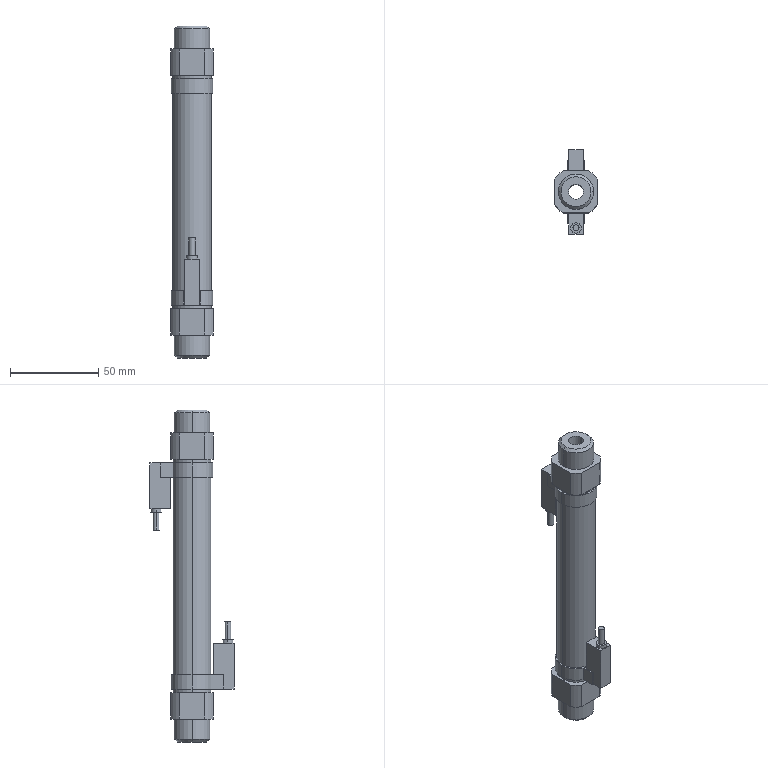Part | STEP file | body_A_CDM2WB20_100_C76_0_ | 1 solid | 97 faces | box 24 x 47.6 x 188 mm | volume 67570 mm3 | plane 49 | cylinder 40 | cone 8 | commonest cylinder face diameters 23.6 x8 28 x8 21.6 x6 3.4 x4 6 x4 8.57 x4